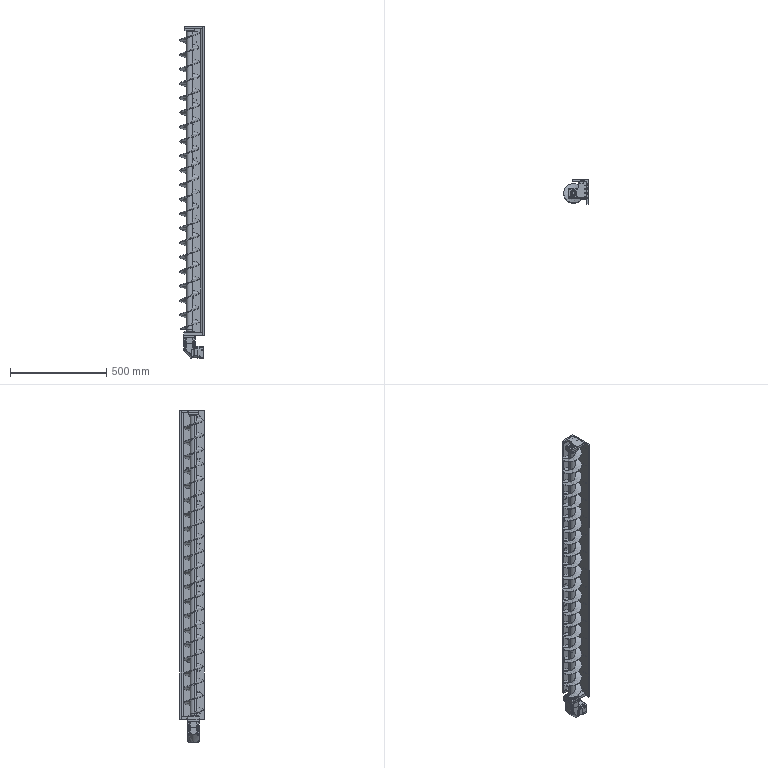Part | SolidWorks | 22 solids | 1040 faces | box 127 x 125 x 1722 mm | volume 4062488 mm3 | cylinder 554 | plane 298 | cone 111 | spline 53 | torus 24 | commonest cylinder face diameters 4.2 x190 5.5 x40 10.1 x30 10 x28 69 x26 3.3 x18